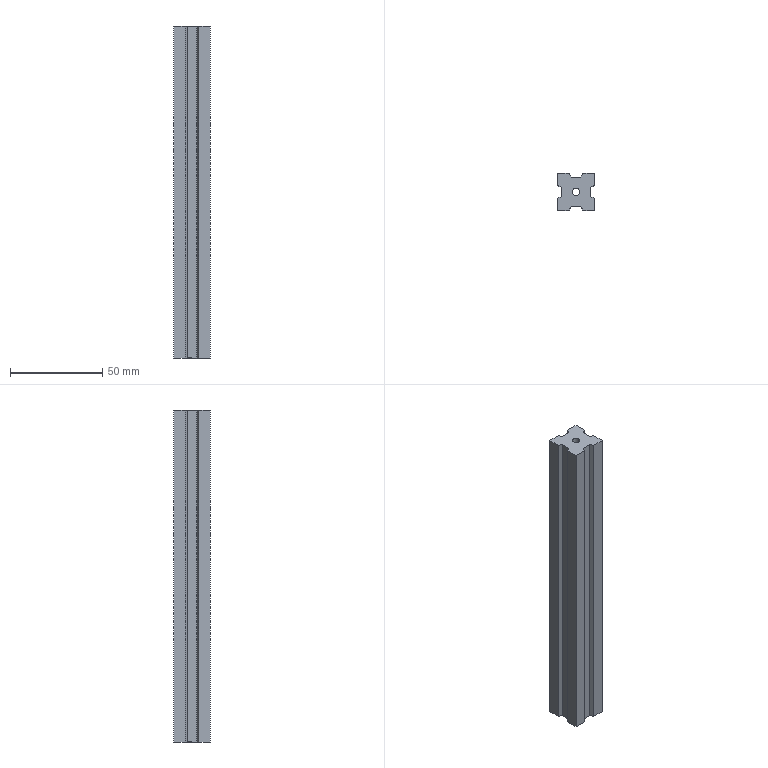Part | SolidWorks | features CirPattern 1, Extrusion 1, ICE 1 | 1 solid | 24 faces | box 20 x 20 x 180 mm | volume 60635 mm3 | plane 22 | cylinder 2 | commonest cylinder face diameters 3.889 x2
STEP:
#1=CARTESIAN_POINT('',(-1.944,0.,90.));
#2=VERTEX_POINT('',#1);
#3=CARTESIAN_POINT('',(1.944,0.,90.));
#4=VERTEX_POINT('',#3);
#5=CARTESIAN_POINT('',(0.,0.,90.));
#6=DIRECTION('',(0.,0.,1.));
#7=DIRECTION('',(1.,0.,0.));
#8=AXIS2_PLACEMENT_3D('',#5,#6,#7);
#9=CIRCLE('',#8,1.944);
#10=EDGE_CURVE('',#2,#4,#9,.T.);
#11=ORIENTED_EDGE('',*,*,#10,.T.);
#12=CARTESIAN_POINT('',(1.944,0.,-90.));
#13=VERTEX_POINT('',#12);
#14=CARTESIAN_POINT('',(1.944,0.,90.));
#15=DIRECTION('',(0.,0.,-1.));
#16=VECTOR('',#15,1000.);
#17=LINE('',#14,#16);
#18=EDGE_CURVE('',#4,#13,#17,.T.);
#19=ORIENTED_EDGE('',*,*,#18,.T.);
#20=CARTESIAN_POINT('',(-1.944,0.,-90.));
#21=VERTEX_POINT('',#20);
#22=CARTESIAN_POINT('',(0.,0.,-90.));
#23=DIRECTION('',(0.,0.,1.));
#24=DIRECTION('',(1.,0.,0.));
#25=AXIS2_PLACEMENT_3D('',#22,#23,#24);
#26=CIRCLE('',#25,1.944);
#27=EDGE_CURVE('',#21,#13,#26,.T.);
#28=ORIENTED_EDGE('',*,*,#27,.F.);
#29=CARTESIAN_POINT('',(-1.944,0.,90.));
#30=DIRECTION('',(0.,0.,-1.));
#31=VECTOR('',#30,1000.);
#32=LINE('',#29,#31);
#33=EDGE_CURVE('',#2,#21,#32,.T.);
#34=ORIENTED_EDGE('',*,*,#33,.F.);
#35=EDGE_LOOP('',(#11,#19,#28,#34));
#36=FACE_OUTER_BOUND('',#35,.T.);
#37=CARTESIAN_POINT('',(0.,0.,90.));
#38=DIRECTION('',(0.,0.,-1.));
#39=DIRECTION('',(-1.,0.,0.));
#40=AXIS2_PLACEMENT_3D('',#37,#38,#39);
#41=CYLINDRICAL_SURFACE('',#40,1.944);
#42=ADVANCED_FACE('',(#36),#41,.F.);
#43=CARTESIAN_POINT('',(-10.,3.694,90.));
#44=VERTEX_POINT('',#43);
#45=CARTESIAN_POINT('',(-10.,3.694,-90.));
#46=VERTEX_POINT('',#45);
#47=CARTESIAN_POINT('',(-10.,3.694,317.761));
#48=DIRECTION('',(0.,0.,-1.));
#49=VECTOR('',#48,1000.);
#50=LINE('',#47,#49);
#51=EDGE_CURVE('',#44,#46,#50,.T.);
#52=ORIENTED_EDGE('',*,*,#51,.F.);
#53=CARTESIAN_POINT('',(-10.,10.,90.));
#54=VERTEX_POINT('',#53);
#55=CARTESIAN_POINT('',(-10.,-10.,90.));
#56=DIRECTION('',(0.,-1.,0.));
#57=VECTOR('',#56,1000.);
#58=LINE('',#55,#57);
#59=EDGE_CURVE('',#54,#44,#58,.T.);
#60=ORIENTED_EDGE('',*,*,#59,.F.);
#61=CARTESIAN_POINT('',(-10.,10.,-90.));
#62=VERTEX_POINT('',#61);
#63=CARTESIAN_POINT('',(-10.,10.,90.));
#64=DIRECTION('',(0.,0.,-1.));
#65=VECTOR('',#64,1000.);
#66=LINE('',#63,#65);
#67=EDGE_CURVE('',#54,#62,#66,.T.);
#68=ORIENTED_EDGE('',*,*,#67,.T.);
#69=CARTESIAN_POINT('',(-10.,-10.,-90.));
#70=DIRECTION('',(0.,-1.,0.));
#71=VECTOR('',#70,1000.);
#72=LINE('',#69,#71);
#73=EDGE_CURVE('',#62,#46,#72,.T.);
#74=ORIENTED_EDGE('',*,*,#73,.T.);
#75=EDGE_LOOP('',(#52,#60,#68,#74));
#76=FACE_OUTER_BOUND('',#75,.T.);
#77=CARTESIAN_POINT('',(-10.,-10.,90.));
#78=DIRECTION('',(1.,0.,0.));
#79=DIRECTION('',(0.,0.,-1.));
#80=AXIS2_PLACEMENT_3D('',#77,#78,#79);
#81=PLANE('',#80);
#82=ADVANCED_FACE('',(#76),#81,.F.);
#83=ORIENTED_EDGE('',*,*,#10,.F.);
#84=CARTESIAN_POINT('',(0.,0.,90.));
#85=DIRECTION('',(0.,0.,1.));
#86=DIRECTION('',(1.,0.,0.));
#87=AXIS2_PLACEMENT_3D('',#84,#85,#86);
#88=CIRCLE('',#87,1.944);
#89=EDGE_CURVE('',#4,#2,#88,.T.);
#90=ORIENTED_EDGE('',*,*,#89,.F.);
#91=EDGE_LOOP('',(#83,#90));
#92=FACE_BOUND('',#91,.T.);
#93=CARTESIAN_POINT('',(-7.931,2.5,90.));
#94=VERTEX_POINT('',#93);
#95=CARTESIAN_POINT('',(-7.931,-2.5,90.));
#96=VERTEX_POINT('',#95);
#97=CARTESIAN_POINT('',(-7.931,0.,90.));
#98=DIRECTION('',(0.,-1.,0.));
#99=VECTOR('',#98,1000.);
#100=LINE('',#97,#99);
#101=EDGE_CURVE('',#94,#96,#100,.T.);
#102=ORIENTED_EDGE('',*,*,#101,.T.);
#103=CARTESIAN_POINT('',(-10.,-3.694,90.));
#104=VERTEX_POINT('',#103);
#105=CARTESIAN_POINT('',(-0.9003,1.559,90.));
#106=DIRECTION('',(-0.866,-0.5,0.));
#107=VECTOR('',#106,1000.);
#108=LINE('',#105,#107);
#109=EDGE_CURVE('',#96,#104,#108,.T.);
#110=ORIENTED_EDGE('',*,*,#109,.T.);
#111=CARTESIAN_POINT('',(-10.,-10.,90.));
#112=VERTEX_POINT('',#111);
#113=CARTESIAN_POINT('',(-10.,-10.,90.));
#114=DIRECTION('',(0.,-1.,0.));
#115=VECTOR('',#114,1000.);
#116=LINE('',#113,#115);
#117=EDGE_CURVE('',#104,#112,#116,.T.);
#118=ORIENTED_EDGE('',*,*,#117,.T.);
#119=CARTESIAN_POINT('',(-3.694,-10.,90.));
#120=VERTEX_POINT('',#119);
#121=CARTESIAN_POINT('',(10.,-10.,90.));
#122=DIRECTION('',(1.,0.,0.));
#123=VECTOR('',#122,1000.);
#124=LINE('',#121,#123);
#125=EDGE_CURVE('',#112,#120,#124,.T.);
#126=ORIENTED_EDGE('',*,*,#125,.T.);
#127=CARTESIAN_POINT('',(-2.5,-7.931,90.));
#128=VERTEX_POINT('',#127);
#129=CARTESIAN_POINT('',(1.559,-0.9003,90.));
#130=DIRECTION('',(0.5,0.866,0.));
#131=VECTOR('',#130,1000.);
#132=LINE('',#129,#131);
#133=EDGE_CURVE('',#120,#128,#132,.T.);
#134=ORIENTED_EDGE('',*,*,#133,.T.);
#135=CARTESIAN_POINT('',(2.5,-7.931,90.));
#136=VERTEX_POINT('',#135);
#137=CARTESIAN_POINT('',(0.,-7.931,90.));
#138=DIRECTION('',(1.,0.,0.));
#139=VECTOR('',#138,1000.);
#140=LINE('',#137,#139);
#141=EDGE_CURVE('',#128,#136,#140,.T.);
#142=ORIENTED_EDGE('',*,*,#141,.T.);
#143=CARTESIAN_POINT('',(3.694,-10.,90.));
#144=VERTEX_POINT('',#143);
#145=CARTESIAN_POINT('',(-1.559,-0.9003,90.));
#146=DIRECTION('',(0.5,-0.866,0.));
#147=VECTOR('',#146,1000.);
#148=LINE('',#145,#147);
#149=EDGE_CURVE('',#136,#144,#148,.T.);
#150=ORIENTED_EDGE('',*,*,#149,.T.);
#151=CARTESIAN_POINT('',(10.,-10.,90.));
#152=VERTEX_POINT('',#151);
#153=CARTESIAN_POINT('',(10.,-10.,90.));
#154=DIRECTION('',(1.,0.,0.));
#155=VECTOR('',#154,1000.);
#156=LINE('',#153,#155);
#157=EDGE_CURVE('',#144,#152,#156,.T.);
#158=ORIENTED_EDGE('',*,*,#157,.T.);
#159=CARTESIAN_POINT('',(10.,-3.694,90.));
#160=VERTEX_POINT('',#159);
#161=CARTESIAN_POINT('',(10.,-10.,90.));
#162=DIRECTION('',(0.,1.,0.));
#163=VECTOR('',#162,1000.);
#164=LINE('',#161,#163);
#165=EDGE_CURVE('',#152,#160,#164,.T.);
#166=ORIENTED_EDGE('',*,*,#165,.T.);
#167=CARTESIAN_POINT('',(7.931,-2.5,90.));
#168=VERTEX_POINT('',#167);
#169=CARTESIAN_POINT('',(0.9003,1.559,90.));
#170=DIRECTION('',(-0.866,0.5,0.));
#171=VECTOR('',#170,1000.);
#172=LINE('',#169,#171);
#173=EDGE_CURVE('',#160,#168,#172,.T.);
#174=ORIENTED_EDGE('',*,*,#173,.T.);
#175=CARTESIAN_POINT('',(7.931,2.5,90.));
#176=VERTEX_POINT('',#175);
#177=CARTESIAN_POINT('',(7.931,0.,90.));
#178=DIRECTION('',(0.,1.,0.));
#179=VECTOR('',#178,1000.);
#180=LINE('',#177,#179);
#181=EDGE_CURVE('',#168,#176,#180,.T.);
#182=ORIENTED_EDGE('',*,*,#181,.T.);
#183=CARTESIAN_POINT('',(10.,3.694,90.));
#184=VERTEX_POINT('',#183);
#185=CARTESIAN_POINT('',(0.9003,-1.559,90.));
#186=DIRECTION('',(0.866,0.5,0.));
#187=VECTOR('',#186,1000.);
#188=LINE('',#185,#187);
#189=EDGE_CURVE('',#176,#184,#188,.T.);
#190=ORIENTED_EDGE('',*,*,#189,.T.);
#191=CARTESIAN_POINT('',(10.,10.,90.));
#192=VERTEX_POINT('',#191);
#193=CARTESIAN_POINT('',(10.,-10.,90.));
#194=DIRECTION('',(0.,1.,0.));
#195=VECTOR('',#194,1000.);
#196=LINE('',#193,#195);
#197=EDGE_CURVE('',#184,#192,#196,.T.);
#198=ORIENTED_EDGE('',*,*,#197,.T.);
#199=CARTESIAN_POINT('',(3.694,10.,90.));
#200=VERTEX_POINT('',#199);
#201=CARTESIAN_POINT('',(10.,10.,90.));
#202=DIRECTION('',(-1.,0.,0.));
#203=VECTOR('',#202,1000.);
#204=LINE('',#201,#203);
#205=EDGE_CURVE('',#192,#200,#204,.T.);
#206=ORIENTED_EDGE('',*,*,#205,.T.);
#207=CARTESIAN_POINT('',(2.5,7.931,90.));
#208=VERTEX_POINT('',#207);
#209=CARTESIAN_POINT('',(-1.559,0.9003,90.));
#210=DIRECTION('',(-0.5,-0.866,0.));
#211=VECTOR('',#210,1000.);
#212=LINE('',#209,#211);
#213=EDGE_CURVE('',#200,#208,#212,.T.);
#214=ORIENTED_EDGE('',*,*,#213,.T.);
#215=CARTESIAN_POINT('',(-2.5,7.931,90.));
#216=VERTEX_POINT('',#215);
#217=CARTESIAN_POINT('',(0.,7.931,90.));
#218=DIRECTION('',(-1.,0.,0.));
#219=VECTOR('',#218,1000.);
#220=LINE('',#217,#219);
#221=EDGE_CURVE('',#208,#216,#220,.T.);
#222=ORIENTED_EDGE('',*,*,#221,.T.);
#223=CARTESIAN_POINT('',(-3.694,10.,90.));
#224=VERTEX_POINT('',#223);
#225=CARTESIAN_POINT('',(1.559,0.9003,90.));
#226=DIRECTION('',(-0.5,0.866,0.));
#227=VECTOR('',#226,1000.);
#228=LINE('',#225,#227);
#229=EDGE_CURVE('',#216,#224,#228,.T.);
#230=ORIENTED_EDGE('',*,*,#229,.T.);
#231=CARTESIAN_POINT('',(10.,10.,90.));
#232=DIRECTION('',(-1.,0.,0.));
#233=VECTOR('',#232,1000.);
#234=LINE('',#231,#233);
#235=EDGE_CURVE('',#224,#54,#234,.T.);
#236=ORIENTED_EDGE('',*,*,#235,.T.);
#237=ORIENTED_EDGE('',*,*,#59,.T.);
#238=CARTESIAN_POINT('',(-0.9003,-1.559,90.));
#239=DIRECTION('',(0.866,-0.5,0.));
#240=VECTOR('',#239,1000.);
#241=LINE('',#238,#240);
#242=EDGE_CURVE('',#44,#94,#241,.T.);
#243=ORIENTED_EDGE('',*,*,#242,.T.);
#244=EDGE_LOOP('',(#102,#110,#118,#126,#134,#142,#150,#158,#166,#174,#182,#190,#198,#206,#214,#222,#230,#236,#237,#243));
#245=FACE_OUTER_BOUND('',#244,.T.);
#246=CARTESIAN_POINT('',(0.,0.,90.));
#247=DIRECTION('',(0.,0.,1.));
#248=DIRECTION('',(1.,0.,0.));
#249=AXIS2_PLACEMENT_3D('',#246,#247,#248);
#250=PLANE('',#249);
#251=ADVANCED_FACE('',(#92,#245),#250,.T.);
#252=ORIENTED_EDGE('',*,*,#27,.T.);
#253=CARTESIAN_POINT('',(0.,0.,-90.));
#254=DIRECTION('',(0.,0.,1.));
#255=DIRECTION('',(1.,0.,0.));
#256=AXIS2_PLACEMENT_3D('',#253,#254,#255);
#257=CIRCLE('',#256,1.944);
#258=EDGE_CURVE('',#13,#21,#257,.T.);
#259=ORIENTED_EDGE('',*,*,#258,.T.);
#260=EDGE_LOOP('',(#252,#259));
#261=FACE_BOUND('',#260,.T.);
#262=CARTESIAN_POINT('',(-7.931,-2.5,-90.));
#263=VERTEX_POINT('',#262);
#264=CARTESIAN_POINT('',(-10.,-3.694,-90.));
#265=VERTEX_POINT('',#264);
#266=CARTESIAN_POINT('',(-0.9003,1.559,-90.));
#267=DIRECTION('',(-0.866,-0.5,0.));
#268=VECTOR('',#267,1000.);
#269=LINE('',#266,#268);
#270=EDGE_CURVE('',#263,#265,#269,.T.);
#271=ORIENTED_EDGE('',*,*,#270,.F.);
#272=CARTESIAN_POINT('',(-7.931,2.5,-90.));
#273=VERTEX_POINT('',#272);
#274=CARTESIAN_POINT('',(-7.931,0.,-90.));
#275=DIRECTION('',(0.,-1.,0.));
#276=VECTOR('',#275,1000.);
#277=LINE('',#274,#276);
#278=EDGE_CURVE('',#273,#263,#277,.T.);
#279=ORIENTED_EDGE('',*,*,#278,.F.);
#280=CARTESIAN_POINT('',(-0.9003,-1.559,-90.));
#281=DIRECTION('',(0.866,-0.5,0.));
#282=VECTOR('',#281,1000.);
#283=LINE('',#280,#282);
#284=EDGE_CURVE('',#46,#273,#283,.T.);
#285=ORIENTED_EDGE('',*,*,#284,.F.);
#286=ORIENTED_EDGE('',*,*,#73,.F.);
#287=CARTESIAN_POINT('',(-3.694,10.,-90.));
#288=VERTEX_POINT('',#287);
#289=CARTESIAN_POINT('',(10.,10.,-90.));
#290=DIRECTION('',(-1.,0.,0.));
#291=VECTOR('',#290,1000.);
#292=LINE('',#289,#291);
#293=EDGE_CURVE('',#288,#62,#292,.T.);
#294=ORIENTED_EDGE('',*,*,#293,.F.);
#295=CARTESIAN_POINT('',(-2.5,7.931,-90.));
#296=VERTEX_POINT('',#295);
#297=CARTESIAN_POINT('',(1.559,0.9003,-90.));
#298=DIRECTION('',(-0.5,0.866,0.));
#299=VECTOR('',#298,1000.);
#300=LINE('',#297,#299);
#301=EDGE_CURVE('',#296,#288,#300,.T.);
#302=ORIENTED_EDGE('',*,*,#301,.F.);
#303=CARTESIAN_POINT('',(2.5,7.931,-90.));
#304=VERTEX_POINT('',#303);
#305=CARTESIAN_POINT('',(0.,7.931,-90.));
#306=DIRECTION('',(-1.,0.,0.));
#307=VECTOR('',#306,1000.);
#308=LINE('',#305,#307);
#309=EDGE_CURVE('',#304,#296,#308,.T.);
#310=ORIENTED_EDGE('',*,*,#309,.F.);
#311=CARTESIAN_POINT('',(3.694,10.,-90.));
#312=VERTEX_POINT('',#311);
#313=CARTESIAN_POINT('',(-1.559,0.9003,-90.));
#314=DIRECTION('',(-0.5,-0.866,0.));
#315=VECTOR('',#314,1000.);
#316=LINE('',#313,#315);
#317=EDGE_CURVE('',#312,#304,#316,.T.);
#318=ORIENTED_EDGE('',*,*,#317,.F.);
#319=CARTESIAN_POINT('',(10.,10.,-90.));
#320=VERTEX_POINT('',#319);
#321=CARTESIAN_POINT('',(10.,10.,-90.));
#322=DIRECTION('',(-1.,0.,0.));
#323=VECTOR('',#322,1000.);
#324=LINE('',#321,#323);
#325=EDGE_CURVE('',#320,#312,#324,.T.);
#326=ORIENTED_EDGE('',*,*,#325,.F.);
#327=CARTESIAN_POINT('',(10.,3.694,-90.));
#328=VERTEX_POINT('',#327);
#329=CARTESIAN_POINT('',(10.,-10.,-90.));
#330=DIRECTION('',(0.,1.,0.));
#331=VECTOR('',#330,1000.);
#332=LINE('',#329,#331);
#333=EDGE_CURVE('',#328,#320,#332,.T.);
#334=ORIENTED_EDGE('',*,*,#333,.F.);
#335=CARTESIAN_POINT('',(7.931,2.5,-90.));
#336=VERTEX_POINT('',#335);
#337=CARTESIAN_POINT('',(0.9003,-1.559,-90.));
#338=DIRECTION('',(0.866,0.5,0.));
#339=VECTOR('',#338,1000.);
#340=LINE('',#337,#339);
#341=EDGE_CURVE('',#336,#328,#340,.T.);
#342=ORIENTED_EDGE('',*,*,#341,.F.);
#343=CARTESIAN_POINT('',(7.931,-2.5,-90.));
#344=VERTEX_POINT('',#343);
#345=CARTESIAN_POINT('',(7.931,0.,-90.));
#346=DIRECTION('',(0.,1.,0.));
#347=VECTOR('',#346,1000.);
#348=LINE('',#345,#347);
#349=EDGE_CURVE('',#344,#336,#348,.T.);
#350=ORIENTED_EDGE('',*,*,#349,.F.);
#351=CARTESIAN_POINT('',(10.,-3.694,-90.));
#352=VERTEX_POINT('',#351);
#353=CARTESIAN_POINT('',(0.9003,1.559,-90.));
#354=DIRECTION('',(-0.866,0.5,0.));
#355=VECTOR('',#354,1000.);
#356=LINE('',#353,#355);
#357=EDGE_CURVE('',#352,#344,#356,.T.);
#358=ORIENTED_EDGE('',*,*,#357,.F.);
#359=CARTESIAN_POINT('',(10.,-10.,-90.));
#360=VERTEX_POINT('',#359);
#361=CARTESIAN_POINT('',(10.,-10.,-90.));
#362=DIRECTION('',(0.,1.,0.));
#363=VECTOR('',#362,1000.);
#364=LINE('',#361,#363);
#365=EDGE_CURVE('',#360,#352,#364,.T.);
#366=ORIENTED_EDGE('',*,*,#365,.F.);
#367=CARTESIAN_POINT('',(3.694,-10.,-90.));
#368=VERTEX_POINT('',#367);
#369=CARTESIAN_POINT('',(10.,-10.,-90.));
#370=DIRECTION('',(1.,0.,0.));
#371=VECTOR('',#370,1000.);
#372=LINE('',#369,#371);
#373=EDGE_CURVE('',#368,#360,#372,.T.);
#374=ORIENTED_EDGE('',*,*,#373,.F.);
#375=CARTESIAN_POINT('',(2.5,-7.931,-90.));
#376=VERTEX_POINT('',#375);
#377=CARTESIAN_POINT('',(-1.559,-0.9003,-90.));
#378=DIRECTION('',(0.5,-0.866,0.));
#379=VECTOR('',#378,1000.);
#380=LINE('',#377,#379);
#381=EDGE_CURVE('',#376,#368,#380,.T.);
#382=ORIENTED_EDGE('',*,*,#381,.F.);
#383=CARTESIAN_POINT('',(-2.5,-7.931,-90.));
#384=VERTEX_POINT('',#383);
#385=CARTESIAN_POINT('',(0.,-7.931,-90.));
#386=DIRECTION('',(1.,0.,0.));
#387=VECTOR('',#386,1000.);
#388=LINE('',#385,#387);
#389=EDGE_CURVE('',#384,#376,#388,.T.);
#390=ORIENTED_EDGE('',*,*,#389,.F.);
#391=CARTESIAN_POINT('',(-3.694,-10.,-90.));
#392=VERTEX_POINT('',#391);
#393=CARTESIAN_POINT('',(1.559,-0.9003,-90.));
#394=DIRECTION('',(0.5,0.866,0.));
#395=VECTOR('',#394,1000.);
#396=LINE('',#393,#395);
#397=EDGE_CURVE('',#392,#384,#396,.T.);
#398=ORIENTED_EDGE('',*,*,#397,.F.);
#399=CARTESIAN_POINT('',(-10.,-10.,-90.));
#400=VERTEX_POINT('',#399);
#401=CARTESIAN_POINT('',(10.,-10.,-90.));
#402=DIRECTION('',(1.,0.,0.));
#403=VECTOR('',#402,1000.);
#404=LINE('',#401,#403);
#405=EDGE_CURVE('',#400,#392,#404,.T.);
#406=ORIENTED_EDGE('',*,*,#405,.F.);
#407=CARTESIAN_POINT('',(-10.,-10.,-90.));
#408=DIRECTION('',(0.,-1.,0.));
#409=VECTOR('',#408,1000.);
#410=LINE('',#407,#409);
#411=EDGE_CURVE('',#265,#400,#410,.T.);
#412=ORIENTED_EDGE('',*,*,#411,.F.);
#413=EDGE_LOOP('',(#271,#279,#285,#286,#294,#302,#310,#318,#326,#334,#342,#350,#358,#366,#374,#382,#390,#398,#406,#412));
#414=FACE_OUTER_BOUND('',#413,.T.);
#415=CARTESIAN_POINT('',(0.,0.,-90.));
#416=DIRECTION('',(0.,0.,1.));
#417=DIRECTION('',(1.,0.,0.));
#418=AXIS2_PLACEMENT_3D('',#415,#416,#417);
#419=PLANE('',#418);
#420=ADVANCED_FACE('',(#261,#414),#419,.F.);
#421=CARTESIAN_POINT('',(-3.694,-10.,317.761));
#422=DIRECTION('',(0.,0.,-1.));
#423=VECTOR('',#422,1000.);
#424=LINE('',#421,#423);
#425=EDGE_CURVE('',#120,#392,#424,.T.);
#426=ORIENTED_EDGE('',*,*,#425,.F.);
#427=ORIENTED_EDGE('',*,*,#125,.F.);
#428=CARTESIAN_POINT('',(-10.,-10.,90.));
#429=DIRECTION('',(0.,0.,-1.));
#430=VECTOR('',#429,1000.);
#431=LINE('',#428,#430);
#432=EDGE_CURVE('',#112,#400,#431,.T.);
#433=ORIENTED_EDGE('',*,*,#432,.T.);
#434=ORIENTED_EDGE('',*,*,#405,.T.);
#435=EDGE_LOOP('',(#426,#427,#433,#434));
#436=FACE_OUTER_BOUND('',#435,.T.);
#437=CARTESIAN_POINT('',(10.,-10.,90.));
#438=DIRECTION('',(0.,1.,0.));
#439=DIRECTION('',(-1.,0.,0.));
#440=AXIS2_PLACEMENT_3D('',#437,#438,#439);
#441=PLANE('',#440);
#442=ADVANCED_FACE('',(#436),#441,.F.);
#443=CARTESIAN_POINT('',(10.,-3.694,317.761));
#444=DIRECTION('',(0.,0.,-1.));
#445=VECTOR('',#444,1000.);
#446=LINE('',#443,#445);
#447=EDGE_CURVE('',#160,#352,#446,.T.);
#448=ORIENTED_EDGE('',*,*,#447,.F.);
#449=ORIENTED_EDGE('',*,*,#165,.F.);
#450=CARTESIAN_POINT('',(10.,-10.,90.));
#451=DIRECTION('',(0.,0.,-1.));
#452=VECTOR('',#451,1000.);
#453=LINE('',#450,#452);
#454=EDGE_CURVE('',#152,#360,#453,.T.);
#455=ORIENTED_EDGE('',*,*,#454,.T.);
#456=ORIENTED_EDGE('',*,*,#365,.T.);
#457=EDGE_LOOP('',(#448,#449,#455,#456));
#458=FACE_OUTER_BOUND('',#457,.T.);
#459=CARTESIAN_POINT('',(10.,-10.,90.));
#460=DIRECTION('',(-1.,0.,0.));
#461=DIRECTION('',(0.,0.,1.));
#462=AXIS2_PLACEMENT_3D('',#459,#460,#461);
#463=PLANE('',#462);
#464=ADVANCED_FACE('',(#458),#463,.F.);
#465=CARTESIAN_POINT('',(3.694,10.,317.761));
#466=DIRECTION('',(0.,0.,-1.));
#467=VECTOR('',#466,1000.);
#468=LINE('',#465,#467);
#469=EDGE_CURVE('',#200,#312,#468,.T.);
#470=ORIENTED_EDGE('',*,*,#469,.F.);
#471=ORIENTED_EDGE('',*,*,#205,.F.);
#472=CARTESIAN_POINT('',(10.,10.,90.));
#473=DIRECTION('',(0.,0.,-1.));
#474=VECTOR('',#473,1000.);
#475=LINE('',#472,#474);
#476=EDGE_CURVE('',#192,#320,#475,.T.);
#477=ORIENTED_EDGE('',*,*,#476,.T.);
#478=ORIENTED_EDGE('',*,*,#325,.T.);
#479=EDGE_LOOP('',(#470,#471,#477,#478));
#480=FACE_OUTER_BOUND('',#479,.T.);
#481=CARTESIAN_POINT('',(10.,10.,90.));
#482=DIRECTION('',(0.,-1.,0.));
#483=DIRECTION('',(1.,0.,0.));
#484=AXIS2_PLACEMENT_3D('',#481,#482,#483);
#485=PLANE('',#484);
#486=ADVANCED_FACE('',(#480),#485,.F.);
#487=ORIENTED_EDGE('',*,*,#117,.F.);
#488=CARTESIAN_POINT('',(-10.,-3.694,317.761));
#489=DIRECTION('',(0.,0.,-1.));
#490=VECTOR('',#489,1000.);
#491=LINE('',#488,#490);
#492=EDGE_CURVE('',#104,#265,#491,.T.);
#493=ORIENTED_EDGE('',*,*,#492,.T.);
#494=ORIENTED_EDGE('',*,*,#411,.T.);
#495=ORIENTED_EDGE('',*,*,#432,.F.);
#496=EDGE_LOOP('',(#487,#493,#494,#495));
#497=FACE_OUTER_BOUND('',#496,.T.);
#498=CARTESIAN_POINT('',(-10.,-10.,90.));
#499=DIRECTION('',(1.,0.,0.));
#500=DIRECTION('',(0.,0.,-1.));
#501=AXIS2_PLACEMENT_3D('',#498,#499,#500);
#502=PLANE('',#501);
#503=ADVANCED_FACE('',(#497),#502,.F.);
#504=ORIENTED_EDGE('',*,*,#157,.F.);
#505=CARTESIAN_POINT('',(3.694,-10.,317.761));
#506=DIRECTION('',(0.,0.,-1.));
#507=VECTOR('',#506,1000.);
#508=LINE('',#505,#507);
#509=EDGE_CURVE('',#144,#368,#508,.T.);
#510=ORIENTED_EDGE('',*,*,#509,.T.);
#511=ORIENTED_EDGE('',*,*,#373,.T.);
#512=ORIENTED_EDGE('',*,*,#454,.F.);
#513=EDGE_LOOP('',(#504,#510,#511,#512));
#514=FACE_OUTER_BOUND('',#513,.T.);
#515=CARTESIAN_POINT('',(10.,-10.,90.));
#516=DIRECTION('',(0.,1.,0.));
#517=DIRECTION('',(-1.,0.,0.));
#518=AXIS2_PLACEMENT_3D('',#515,#516,#517);
#519=PLANE('',#518);
#520=ADVANCED_FACE('',(#514),#519,.F.);
#521=ORIENTED_EDGE('',*,*,#197,.F.);
#522=CARTESIAN_POINT('',(10.,3.694,317.761));
#523=DIRECTION('',(0.,0.,-1.));
#524=VECTOR('',#523,1000.);
#525=LINE('',#522,#524);
#526=EDGE_CURVE('',#184,#328,#525,.T.);
#527=ORIENTED_EDGE('',*,*,#526,.T.);
#528=ORIENTED_EDGE('',*,*,#333,.T.);
#529=ORIENTED_EDGE('',*,*,#476,.F.);
#530=EDGE_LOOP('',(#521,#527,#528,#529));
#531=FACE_OUTER_BOUND('',#530,.T.);
#532=CARTESIAN_POINT('',(10.,-10.,90.));
#533=DIRECTION('',(-1.,0.,0.));
#534=DIRECTION('',(0.,0.,1.));
#535=AXIS2_PLACEMENT_3D('',#532,#533,#534);
#536=PLANE('',#535);
#537=ADVANCED_FACE('',(#531),#536,.F.);
#538=ORIENTED_EDGE('',*,*,#235,.F.);
#539=CARTESIAN_POINT('',(-3.694,10.,317.761));
#540=DIRECTION('',(0.,0.,-1.));
#541=VECTOR('',#540,1000.);
#542=LINE('',#539,#541);
#543=EDGE_CURVE('',#224,#288,#542,.T.);
#544=ORIENTED_EDGE('',*,*,#543,.T.);
#545=ORIENTED_EDGE('',*,*,#293,.T.);
#546=ORIENTED_EDGE('',*,*,#67,.F.);
#547=EDGE_LOOP('',(#538,#544,#545,#546));
#548=FACE_OUTER_BOUND('',#547,.T.);
#549=CARTESIAN_POINT('',(10.,10.,90.));
#550=DIRECTION('',(0.,-1.,0.));
#551=DIRECTION('',(1.,0.,0.));
#552=AXIS2_PLACEMENT_3D('',#549,#550,#551);
#553=PLANE('',#552);
#554=ADVANCED_FACE('',(#548),#553,.F.);
#555=ORIENTED_EDGE('',*,*,#18,.F.);
#556=ORIENTED_EDGE('',*,*,#89,.T.);
#557=ORIENTED_EDGE('',*,*,#33,.T.);
#558=ORIENTED_EDGE('',*,*,#258,.F.);
#559=EDGE_LOOP('',(#555,#556,#557,#558));
#560=FACE_OUTER_BOUND('',#559,.T.);
#561=CARTESIAN_POINT('',(0.,0.,90.));
#562=DIRECTION('',(0.,0.,-1.));
#563=DIRECTION('',(-1.,0.,0.));
#564=AXIS2_PLACEMENT_3D('',#561,#562,#563);
#565=CYLINDRICAL_SURFACE('',#564,1.944);
#566=ADVANCED_FACE('',(#560),#565,.F.);
#567=ORIENTED_EDGE('',*,*,#229,.F.);
#568=CARTESIAN_POINT('',(-2.5,7.931,317.761));
#569=DIRECTION('',(0.,0.,-1.));
#570=VECTOR('',#569,1000.);
#571=LINE('',#568,#570);
#572=EDGE_CURVE('',#216,#296,#571,.T.);
#573=ORIENTED_EDGE('',*,*,#572,.T.);
#574=ORIENTED_EDGE('',*,*,#301,.T.);
#575=ORIENTED_EDGE('',*,*,#543,.F.);
#576=EDGE_LOOP('',(#567,#573,#574,#575));
#577=FACE_OUTER_BOUND('',#576,.T.);
#578=CARTESIAN_POINT('',(-3.694,10.,317.761));
#579=DIRECTION('',(0.866,0.5,0.));
#580=DIRECTION('',(-0.5,0.866,0.));
#581=AXIS2_PLACEMENT_3D('',#578,#579,#580);
#582=PLANE('',#581);
#583=ADVANCED_FACE('',(#577),#582,.T.);
#584=ORIENTED_EDGE('',*,*,#221,.F.);
#585=CARTESIAN_POINT('',(2.5,7.931,317.761));
#586=DIRECTION('',(0.,0.,-1.));
#587=VECTOR('',#586,1000.);
#588=LINE('',#585,#587);
#589=EDGE_CURVE('',#208,#304,#588,.T.);
#590=ORIENTED_EDGE('',*,*,#589,.T.);
#591=ORIENTED_EDGE('',*,*,#309,.T.);
#592=ORIENTED_EDGE('',*,*,#572,.F.);
#593=EDGE_LOOP('',(#584,#590,#591,#592));
#594=FACE_OUTER_BOUND('',#593,.T.);
#595=CARTESIAN_POINT('',(-2.5,7.931,317.761));
#596=DIRECTION('',(0.,1.,0.));
#597=DIRECTION('',(0.,0.,1.));
#598=AXIS2_PLACEMENT_3D('',#595,#596,#597);
#599=PLANE('',#598);
#600=ADVANCED_FACE('',(#594),#599,.T.);
#601=ORIENTED_EDGE('',*,*,#213,.F.);
#602=ORIENTED_EDGE('',*,*,#469,.T.);
#603=ORIENTED_EDGE('',*,*,#317,.T.);
#604=ORIENTED_EDGE('',*,*,#589,.F.);
#605=EDGE_LOOP('',(#601,#602,#603,#604));
#606=FACE_OUTER_BOUND('',#605,.T.);
#607=CARTESIAN_POINT('',(2.5,7.931,317.761));
#608=DIRECTION('',(-0.866,0.5,0.));
#609=DIRECTION('',(-0.5,-0.866,0.));
#610=AXIS2_PLACEMENT_3D('',#607,#608,#609);
#611=PLANE('',#610);
#612=ADVANCED_FACE('',(#606),#611,.T.);
#613=ORIENTED_EDGE('',*,*,#189,.F.);
#614=CARTESIAN_POINT('',(7.931,2.5,317.761));
#615=DIRECTION('',(0.,0.,-1.));
#616=VECTOR('',#615,1000.);
#617=LINE('',#614,#616);
#618=EDGE_CURVE('',#176,#336,#617,.T.);
#619=ORIENTED_EDGE('',*,*,#618,.T.);
#620=ORIENTED_EDGE('',*,*,#341,.T.);
#621=ORIENTED_EDGE('',*,*,#526,.F.);
#622=EDGE_LOOP('',(#613,#619,#620,#621));
#623=FACE_OUTER_BOUND('',#622,.T.);
#624=CARTESIAN_POINT('',(10.,3.694,317.761));
#625=DIRECTION('',(0.5,-0.866,0.));
#626=DIRECTION('',(0.866,0.5,0.));
#627=AXIS2_PLACEMENT_3D('',#624,#625,#626);
#628=PLANE('',#627);
#629=ADVANCED_FACE('',(#623),#628,.T.);
#630=ORIENTED_EDGE('',*,*,#181,.F.);
#631=CARTESIAN_POINT('',(7.931,-2.5,317.761));
#632=DIRECTION('',(0.,0.,-1.));
#633=VECTOR('',#632,1000.);
#634=LINE('',#631,#633);
#635=EDGE_CURVE('',#168,#344,#634,.T.);
#636=ORIENTED_EDGE('',*,*,#635,.T.);
#637=ORIENTED_EDGE('',*,*,#349,.T.);
#638=ORIENTED_EDGE('',*,*,#618,.F.);
#639=EDGE_LOOP('',(#630,#636,#637,#638));
#640=FACE_OUTER_BOUND('',#639,.T.);
#641=CARTESIAN_POINT('',(7.931,2.5,317.761));
#642=DIRECTION('',(1.,0.,0.));
#643=DIRECTION('',(0.,1.,0.));
#644=AXIS2_PLACEMENT_3D('',#641,#642,#643);
#645=PLANE('',#644);
#646=ADVANCED_FACE('',(#640),#645,.T.);
#647=ORIENTED_EDGE('',*,*,#173,.F.);
#648=ORIENTED_EDGE('',*,*,#447,.T.);
#649=ORIENTED_EDGE('',*,*,#357,.T.);
#650=ORIENTED_EDGE('',*,*,#635,.F.);
#651=EDGE_LOOP('',(#647,#648,#649,#650));
#652=FACE_OUTER_BOUND('',#651,.T.);
#653=CARTESIAN_POINT('',(7.931,-2.5,317.761));
#654=DIRECTION('',(0.5,0.866,0.));
#655=DIRECTION('',(-0.866,0.5,0.));
#656=AXIS2_PLACEMENT_3D('',#653,#654,#655);
#657=PLANE('',#656);
#658=ADVANCED_FACE('',(#652),#657,.T.);
#659=ORIENTED_EDGE('',*,*,#149,.F.);
#660=CARTESIAN_POINT('',(2.5,-7.931,317.761));
#661=DIRECTION('',(0.,0.,-1.));
#662=VECTOR('',#661,1000.);
#663=LINE('',#660,#662);
#664=EDGE_CURVE('',#136,#376,#663,.T.);
#665=ORIENTED_EDGE('',*,*,#664,.T.);
#666=ORIENTED_EDGE('',*,*,#381,.T.);
#667=ORIENTED_EDGE('',*,*,#509,.F.);
#668=EDGE_LOOP('',(#659,#665,#666,#667));
#669=FACE_OUTER_BOUND('',#668,.T.);
#670=CARTESIAN_POINT('',(3.694,-10.,317.761));
#671=DIRECTION('',(-0.866,-0.5,0.));
#672=DIRECTION('',(0.5,-0.866,0.));
#673=AXIS2_PLACEMENT_3D('',#670,#671,#672);
#674=PLANE('',#673);
#675=ADVANCED_FACE('',(#669),#674,.T.);
#676=ORIENTED_EDGE('',*,*,#141,.F.);
#677=CARTESIAN_POINT('',(-2.5,-7.931,317.761));
#678=DIRECTION('',(0.,0.,-1.));
#679=VECTOR('',#678,1000.);
#680=LINE('',#677,#679);
#681=EDGE_CURVE('',#128,#384,#680,.T.);
#682=ORIENTED_EDGE('',*,*,#681,.T.);
#683=ORIENTED_EDGE('',*,*,#389,.T.);
#684=ORIENTED_EDGE('',*,*,#664,.F.);
#685=EDGE_LOOP('',(#676,#682,#683,#684));
#686=FACE_OUTER_BOUND('',#685,.T.);
#687=CARTESIAN_POINT('',(2.5,-7.931,317.761));
#688=DIRECTION('',(0.,-1.,0.));
#689=DIRECTION('',(0.,0.,-1.));
#690=AXIS2_PLACEMENT_3D('',#687,#688,#689);
#691=PLANE('',#690);
#692=ADVANCED_FACE('',(#686),#691,.T.);
#693=ORIENTED_EDGE('',*,*,#133,.F.);
#694=ORIENTED_EDGE('',*,*,#425,.T.);
#695=ORIENTED_EDGE('',*,*,#397,.T.);
#696=ORIENTED_EDGE('',*,*,#681,.F.);
#697=EDGE_LOOP('',(#693,#694,#695,#696));
#698=FACE_OUTER_BOUND('',#697,.T.);
#699=CARTESIAN_POINT('',(-2.5,-7.931,317.761));
#700=DIRECTION('',(0.866,-0.5,0.));
#701=DIRECTION('',(0.5,0.866,0.));
#702=AXIS2_PLACEMENT_3D('',#699,#700,#701);
#703=PLANE('',#702);
#704=ADVANCED_FACE('',(#698),#703,.T.);
#705=ORIENTED_EDGE('',*,*,#109,.F.);
#706=CARTESIAN_POINT('',(-7.931,-2.5,317.761));
#707=DIRECTION('',(0.,0.,-1.));
#708=VECTOR('',#707,1000.);
#709=LINE('',#706,#708);
#710=EDGE_CURVE('',#96,#263,#709,.T.);
#711=ORIENTED_EDGE('',*,*,#710,.T.);
#712=ORIENTED_EDGE('',*,*,#270,.T.);
#713=ORIENTED_EDGE('',*,*,#492,.F.);
#714=EDGE_LOOP('',(#705,#711,#712,#713));
#715=FACE_OUTER_BOUND('',#714,.T.);
#716=CARTESIAN_POINT('',(-10.,-3.694,317.761));
#717=DIRECTION('',(-0.5,0.866,0.));
#718=DIRECTION('',(-0.866,-0.5,0.));
#719=AXIS2_PLACEMENT_3D('',#716,#717,#718);
#720=PLANE('',#719);
#721=ADVANCED_FACE('',(#715),#720,.T.);
#722=ORIENTED_EDGE('',*,*,#101,.F.);
#723=CARTESIAN_POINT('',(-7.931,2.5,317.761));
#724=DIRECTION('',(0.,0.,-1.));
#725=VECTOR('',#724,1000.);
#726=LINE('',#723,#725);
#727=EDGE_CURVE('',#94,#273,#726,.T.);
#728=ORIENTED_EDGE('',*,*,#727,.T.);
#729=ORIENTED_EDGE('',*,*,#278,.T.);
#730=ORIENTED_EDGE('',*,*,#710,.F.);
#731=EDGE_LOOP('',(#722,#728,#729,#730));
#732=FACE_OUTER_BOUND('',#731,.T.);
#733=CARTESIAN_POINT('',(-7.931,-2.5,317.761));
#734=DIRECTION('',(-1.,0.,0.));
#735=DIRECTION('',(0.,-1.,0.));
#736=AXIS2_PLACEMENT_3D('',#733,#734,#735);
#737=PLANE('',#736);
#738=ADVANCED_FACE('',(#732),#737,.T.);
#739=ORIENTED_EDGE('',*,*,#242,.F.);
#740=ORIENTED_EDGE('',*,*,#51,.T.);
#741=ORIENTED_EDGE('',*,*,#284,.T.);
#742=ORIENTED_EDGE('',*,*,#727,.F.);
#743=EDGE_LOOP('',(#739,#740,#741,#742));
#744=FACE_OUTER_BOUND('',#743,.T.);
#745=CARTESIAN_POINT('',(-7.931,2.5,317.761));
#746=DIRECTION('',(-0.5,-0.866,0.));
#747=DIRECTION('',(0.866,-0.5,0.));
#748=AXIS2_PLACEMENT_3D('',#745,#746,#747);
#749=PLANE('',#748);
#750=ADVANCED_FACE('',(#744),#749,.T.);
#751=CLOSED_SHELL('',(#42,#82,#251,#420,#442,#464,#486,#503,#520,#537,#554,#566,#583,#600,#612,#629,#646,#658,#675,#692,#704,#721,#738,#750));
#752=MANIFOLD_SOLID_BREP('',#751);
#753=CARTESIAN_POINT('',(0.,0.,0.));
#754=DIRECTION('',(0.,0.,1.));
#755=DIRECTION('',(1.,0.,0.));
#756=AXIS2_PLACEMENT_3D('',#753,#754,#755);
#757=(LENGTH_UNIT()NAMED_UNIT(*)SI_UNIT(.MILLI.,.METRE.));
#758=UNCERTAINTY_MEASURE_WITH_UNIT(LENGTH_MEASURE(0.00001),#757,'','');
#759=(NAMED_UNIT(*)PLANE_ANGLE_UNIT()SI_UNIT($,.RADIAN.));
#760=(NAMED_UNIT(*)SI_UNIT($,.STERADIAN.)SOLID_ANGLE_UNIT());
#761=(GEOMETRIC_REPRESENTATION_CONTEXT(3)GLOBAL_UNCERTAINTY_ASSIGNED_CONTEXT((#758))GLOBAL_UNIT_ASSIGNED_CONTEXT((#757,#759,#760))REPRESENTATION_CONTEXT('',''));
#762=ADVANCED_BREP_SHAPE_REPRESENTATION('',(#752,#756),#761);